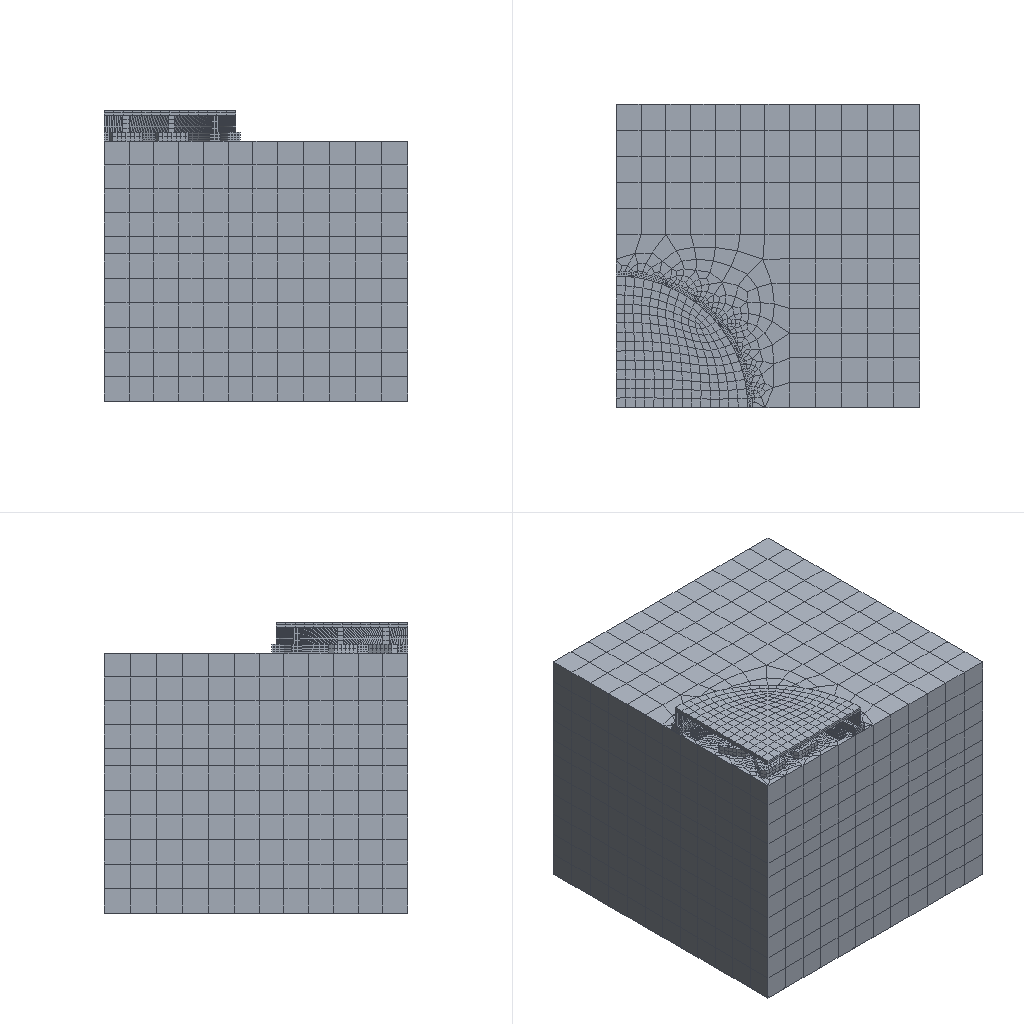Simulation study | abaqus
Set-up summary:
category,name,step,type,value,unit,region
solver,abaqus
solver,version,,,Abaqus/Standard 2020
units,not stated in the deck,,not stated
analysis,deck,,geostatic,geostatic
load_step,geo,geo,geostatic
load_step,load,load,static
load_step,requested,,,2
mesh,nodes,,,48393
mesh,elements,,,38413
element_type,C3D8,,solid,38413
load,load commands in deck,,count,2
bc,support commands in deck,,count,5
material,CANGDI,,in results
material,PILE,,in results
material,SOIL,,in results
check,setup vs results,,match,"per instance, exact: element labels, types and connectivity; labels of the nodes the elements use; coordinates of those nodes at SINGLE_PRECISION in 8 of 9 instance(s)"
Abaqus input file, long lists of numbers shortened:
*Heading
** Job name: Job-2 Model name: Model-1-4D-tiaoshi
** Generated by: Abaqus/CAE 2020
*Preprint, echo=NO, model=NO, history=NO, contact=NO
**
** PARTS
**
*Part, name=cangdi
*Node
      1,           0.,           0.,         0.25
      2,           0.,           0.,          0.5
** (637 more lines like these left out)
*Element, type=C3D8
  1,  72,  92, 320, 220,   1,   2,  22,  41
  2, 220, 320, 321, 221,  41,  22,  23,  40
** (372 more lines like these left out)
*Nset, nset=Set-1, generate
   1,  639,    1
*Elset, elset=Set-1, generate
   1,  374,    1
** Section: cangdi
*Solid Section, elset=Set-1, material=cangdi
,
*End Part
**
*Part, name=fangCT-Pile
*Node
      1,           0.,   1.2,           1.
      2,           0.,           0.,           1.
** (3217 more lines like these left out)
*Element, type=C3D8
   1,  266,  364,  282,  265, 1719, 1817, 1735, 1718
   2,  306,  289,   35,   34, 1759, 1742,  792,  793
** (2346 more lines like these left out)
*Nset, nset=Set-17, generate
    1,  3219,     1
*Elset, elset=Set-17, generate
    1,  2348,     1
** Section: pile
*Solid Section, elset=Set-17, material=pile
,
*End Part
**
*Part, name=huxingCT-pile
*Node
      1,   14.85,           0.,           3.
      2,           0.,   14.85,           3.
** (14026 more lines like these left out)
*Element, type=C3D8
  1,  494, 1649, 7421, 1647,    1,   65, 1423,  278
  2, 1649, 1650, 7422, 7421,   65,   66, 1424, 1423
** (10161 more lines like these left out)
*Nset, nset=Set-13, generate
     1,  14028,      1
*Elset, elset=Set-13, generate
     1,  10163,      1
** Section: pile
*Solid Section, elset=Set-13, material=pile
,
*End Part
**
*Part, name=sanjiaoCT-pile
*Node
      1,  0.35, -0.3489,           3.
      2, -0.35, -0.3489,           3.
** (776 more lines like these left out)
*Element, type=C3D8
1,  8,  5, 40, 41,  1,  2, 32, 37
2, 41, 40, 39, 42, 37, 32, 33, 36
** (366 more lines like these left out)
*Nset, nset=Set-5, generate
   1,  778,    1
*Elset, elset=Set-5, generate
   1,  368,    1
** Section: pile
*Solid Section, elset=Set-5, material=pile
,
*End Part
**
*Part, name=soil-1
*Node
      1,          20.,          20.,          39.
      2,           0.,          20.,          39.
** (24174 more lines like these left out)
*Element, type=C3D8
 1,   1,  81, 613, 100,   5, 101, 637, 120
 2,  81,  82, 614, 613, 101, 102, 638, 637
** (21706 more lines like these left out)
*Nset, nset=Set-4, generate
     1,  24176,      1
*Elset, elset=Set-4, generate
     1,  21708,      1
** Section: soil
*Solid Section, elset=Set-4, material=soil
,
*End Part
**
**
** ASSEMBLY
**
*Assembly, name=Assembly
**
*Instance, name=soil-1-1, part=soil-1
*End Instance
**
*Instance, name=cangdi-1, part=cangdi
          0.,           0.,          53.
*End Instance
**
*Instance, name=fangCT-Pile-3, part=fangCT-Pile
0.7,         12.2,          50.
*End Instance
**
*Instance, name=huxingCT-pile-1, part=huxingCT-pile
          0.,           0.,          50.
*End Instance
**
*Instance, name=sanjiaoCT-pile-5, part=sanjiaoCT-pile
         2.5,          2.5,          50.
*End Instance
**
*Instance, name=sanjiaoCT-pile-6, part=sanjiaoCT-pile
         7.8,          2.5,          50.
*End Instance
**
*Instance, name=sanjiaoCT-pile-7, part=sanjiaoCT-pile
2.5, 7.8,          50.
2.5, 7.8,          50., 2.5, 7.8,          51.,         180.
*End Instance
**
*Instance, name=sanjiaoCT-pile-8, part=sanjiaoCT-pile
         7.8,          7.8,          50.
         7.8,          7.8,          50.,          7.8,          7.8,          51.,         180.
*End Instance
**
*Instance, name=fangCT-Pile-4, part=fangCT-Pile
        12.2,          4.3,          50.
        12.2,          4.3,          50.,         12.2,          4.3, 49., 90.
*End Instance
**
*Node
      1,           6.,           6.,         56.5
*Nset, nset=Set-1
 1,
*Nset, nset=Set-2, instance=soil-1-1
   19,   20,   21,   22,   23,   24,   55,   56,   58,  207,  208,  209,  210,  211,  212,  213
  214,  239,  240,  241,  242,  243,  244,  245,  246,  247,  248,  447,  448,  449,  450,  451
** (3 more lines like these left out)
*Elset, elset=Set-2, instance=soil-1-1
   421,   422,   423,   424,   425,   456,   457,   458,   459,   460,   461,   462,   463,   464,   465,   466
   467,   468,   469,   470,   471,   472,   473,   474,   475,  1196,  1490,  1909,  1911,  1920,  2288,  2831
** (2 more lines like these left out)
*Nset, nset=Set-3, instance=soil-1-1
    2,    3,    6,    7,    9,   10,   11,   12,   20,   21,   24,   25,   30,   31,   32,   55
   56,   58,   87,   88,   89,   90,  107,  108,  109,  110,  129,  130,  131,  132,  141,  142
** (8 more lines like these left out)
*Elset, elset=Set-3, instance=soil-1-1
     7,    14,    21,    28,    35,    36,    41,    46,    51,    56,   425,   430,   435,   440,   445,   450
   455,   472,   473,   474,   475,   492,   493,   494,   495,   512,   513,   514,   515,   532,   533,   534
** (6 more lines like these left out)
*Nset, nset=Set-4, instance=soil-1-1
    3,    4,    7,    8,   10,   12,   19,   20,   21,   22,   23,   24,   29,   30,   31,   55
   56,   58,   91,   92,   93,   94,   95,   96,  111,  112,  113,  114,  115,  116,  125,  126
** (8 more lines like these left out)
*Elset, elset=Set-4, instance=soil-1-1
    29,    30,    31,    32,    33,    34,    35,    56,    57,    58,    59,    60,   421,   422,   423,   424
   425,   456,   457,   458,   459,   460,   461,   462,   463,   464,   465,   466,   467,   468,   469,   470
** (6 more lines like these left out)
*Nset, nset=Set-6
 1,
*Nset, nset=Set-7, instance=soil-1-1, generate
     1,  24176,      1
*Elset, elset=Set-7, instance=soil-1-1, generate
     1,  21708,      1
*Nset, nset=Set-10, instance=soil-1-1
    2,    3,    6,    7,    9,   10,   11,   12,   14,   15,   17,   18,   20,   21,   24,   25
   28,   30,   31,   32,   55,   56,   57,   58,   87,   88,   89,   90,  107,  108,  109,  110
** (18 more lines like these left out)
*Elset, elset=Set-10, instance=soil-1-1
     7,    14,    21,    28,    35,    36,    41,    46,    51,    56,    67,    74,    81,    88,    95,   102
   109,   116,   123,   130,   137,   144,   151,   158,   165,   172,   179,   186,   193,   200,   207,   214
** (15 more lines like these left out)
*Nset, nset=Set-11, instance=soil-1-1
    3,    4,    7,    8,   10,   12,   15,   16,   17,   19,   20,   21,   22,   23,   24,   27
   28,   29,   30,   31,   55,   56,   57,   58,   91,   92,   93,   94,   95,   96,  111,  112
** (18 more lines like these left out)
*Elset, elset=Set-11, instance=soil-1-1
    29,    30,    31,    32,    33,    34,    35,    56,    57,    58,    59,    60,    89,    90,    91,    92
    93,    94,    95,   124,   125,   126,   127,   128,   129,   130,   159,   160,   161,   162,   163,   164
** (15 more lines like these left out)
*Nset, nset=Set-12, instance=soil-1-1
   13,   14,   15,   16,   17,   18,   27,   28,   57,  145,  146,  147,  148,  149,  150,  151
  152,  153,  154,  155,  156,  157,  158,  159,  160,  161,  162,  163,  164,  185,  186,  187
** (125 more lines like these left out)
*Elset, elset=Set-12, instance=soil-1-1
    61,    62,    63,    64,    65,    66,    67,    68,    69,    70,    71,    72,    73,    74,    75,    76
    77,    78,    79,    80,    81,    82,    83,    84,    85,    86,    87,    88,    89,    90,    91,    92
** (123 more lines like these left out)
*Nset, nset=Set-13, instance=soil-1-1, generate
     1,  24176,      1
*Elset, elset=Set-13, instance=soil-1-1, generate
     1,  21708,      1
*Nset, nset=Set-14, instance=soil-1-1, generate
     1,  24176,      1
*Elset, elset=Set-14, instance=soil-1-1, generate
     1,  21708,      1
*Nset, nset=m_Set-9
 1,
*Elset, elset=_Surf-zhuding_S2, internal, instance=fangCT-Pile-3, generate
 1829,  1844,     1
*Elset, elset=_Surf-zhuding_S2, internal, instance=fangCT-Pile-4, generate
 1829,  1844,     1
*Elset, elset=_Surf-zhuding_S3, internal, instance=huxingCT-pile-1
   1,   2,   3,   4,   5,   6,   7,   8,   9,  10,  11,  12,  13,  14,  15,  16
  17,  18,  19,  20,  21,  22,  23,  24,  25,  26,  27,  28,  29,  30,  31,  32
** (13 more lines like these left out)
*Elset, elset=_Surf-zhuding_S3, internal, instance=sanjiaoCT-pile-7
 1,
*Elset, elset=_Surf-zhuding_S3, internal, instance=sanjiaoCT-pile-5
 1,
*Elset, elset=_Surf-zhuding_S3, internal, instance=sanjiaoCT-pile-8
 1,
*Elset, elset=_Surf-zhuding_S3, internal, instance=sanjiaoCT-pile-6
 1,
*Surface, type=ELEMENT, name=Surf-zhuding
_Surf-zhuding_S2, S2
_Surf-zhuding_S3, S3
*Elset, elset=_s_Surf-5_S4, internal, instance=cangdi-1, generate
   1,  121,    1
*Elset, elset=_s_Surf-5_S3, internal, instance=cangdi-1, generate
 122,  154,    1
*Elset, elset=_s_Surf-5_S2, internal, instance=cangdi-1, generate
 309,  341,    1
*Surface, type=ELEMENT, name=s_Surf-5
_s_Surf-5_S4, S4
_s_Surf-5_S3, S3
_s_Surf-5_S2, S2
*Elset, elset=_s_Surf-6_S2, internal, instance=soil-1-1, generate
 19863,  21708,      1
*Elset, elset=_s_Surf-6_S4, internal, instance=soil-1-1
 14332, 14347, 14366, 14367, 14381, 14388, 14389, 14427, 14443, 14465, 14472, 14484, 14504, 14515, 14516, 14523
 14531, 14559, 14581, 14596, 14602, 14693, 16178, 16193, 16212, 16213, 16227, 16234, 16235, 16273, 16289, 16311
** (4 more lines like these left out)
*Elset, elset=_s_Surf-6_S6, internal, instance=soil-1-1
 14331, 14352, 14369, 14371, 14372, 14376, 14380, 14382, 14393, 14406, 14407, 14415, 14418, 14449, 14452, 14469
 14475, 14477, 14487, 14506, 14509, 14513, 14519, 14522, 14524, 14601, 14626, 16177, 16198, 16215, 16217, 16218
** (5 more lines like these left out)
*Elset, elset=_s_Surf-6_S3, internal, instance=soil-1-1
 14326, 14354, 14363, 14379, 14390, 14400, 14413, 14433, 14462, 14463, 14534, 14545, 14557, 14570, 14577, 14584
 14620, 14632, 14640, 14656, 14669, 14672, 14679, 14698, 14915, 14944, 16172, 16200, 16209, 16225, 16236, 16246
** (5 more lines like these left out)
*Elset, elset=_s_Surf-6_S5, internal, instance=soil-1-1
 14335, 14343, 14359, 14361, 14365, 14370, 14386, 14391, 14395, 14403, 14421, 14423, 14425, 14431, 14451, 14453
 14466, 14470, 14473, 14478, 14482, 14483, 14486, 14488, 14491, 14498, 14499, 14501, 14507, 14510, 14514, 14518
** (13 more lines like these left out)
*Elset, elset=_s_Surf-6_S1, internal, instance=soil-1-1, generate
 1046,  1096,     1
*Surface, type=ELEMENT, name=s_Surf-6
_s_Surf-6_S2, S2
_s_Surf-6_S4, S4
_s_Surf-6_S6, S6
_s_Surf-6_S3, S3
_s_Surf-6_S5, S5
_s_Surf-6_S1, S1
*Elset, elset=_surf-allpile_S2, internal, instance=fangCT-Pile-3, generate
  871,  1044,     1
*Elset, elset=_surf-allpile_S2, internal, instance=huxingCT-pile-1, generate
 5325,  6287,     1
*Elset, elset=_surf-allpile_S2, internal, instance=sanjiaoCT-pile-7, generate
  55,  104,    1
*Elset, elset=_surf-allpile_S2, internal, instance=fangCT-Pile-4, generate
  871,  1044,     1
*Elset, elset=_surf-allpile_S2, internal, instance=sanjiaoCT-pile-5, generate
  55,  104,    1
*Elset, elset=_surf-allpile_S2, internal, instance=sanjiaoCT-pile-8, generate
  55,  104,    1
*Elset, elset=_surf-allpile_S2, internal, instance=sanjiaoCT-pile-6, generate
  55,  104,    1
*Surface, type=ELEMENT, name=surf-allpile
_surf-allpile_S2, S2
*Elset, elset=_surf-allsoil-p_S6, internal, instance=soil-1-1
   456,   460,   464,   468,   472,   476,   480,   484,   488,   492,   496,   500,   504,   508,   512,   516
   520,   524,   528,   532,   536,   540,   544,   548,   552,   556,   560,   564,   568,   572,   576,   580
** (10 more lines like these left out)
*Elset, elset=_surf-allsoil-p_S2, internal, instance=soil-1-1, generate
 19863,  21708,      1
*Elset, elset=_surf-allsoil-p_S4, internal, instance=soil-1-1
   809,   813,   817,   821,   825,   829,   833,   837,   841,   845,   849,   853,   857,   861,   865,   869
   873,   877,   881,   885,   889,   893,   897,   901,   905, 14332, 14347, 14366, 14367, 14381, 14388, 14389
** (6 more lines like these left out)
*Elset, elset=_surf-allsoil-p_S3, internal, instance=soil-1-1
 14326, 14354, 14363, 14379, 14390, 14400, 14413, 14433, 14462, 14463, 14534, 14545, 14557, 14570, 14577, 14584
 14620, 14632, 14640, 14656, 14669, 14672, 14679, 14698, 14915, 14944, 16172, 16200, 16209, 16225, 16236, 16246
** (5 more lines like these left out)
*Elset, elset=_surf-allsoil-p_S5, internal, instance=soil-1-1
 14335, 14343, 14359, 14361, 14365, 14370, 14386, 14391, 14395, 14403, 14421, 14423, 14425, 14431, 14451, 14453
 14466, 14470, 14473, 14478, 14482, 14483, 14486, 14488, 14491, 14498, 14499, 14501, 14507, 14510, 14514, 14518
** (13 more lines like these left out)
*Elset, elset=_surf-allsoil-p_S1, internal, instance=soil-1-1, generate
 1046,  1096,     1
*Surface, type=ELEMENT, name=surf-allsoil-p
_surf-allsoil-p_S6, S6
_surf-allsoil-p_S2, S2
_surf-allsoil-p_S4, S4
_surf-allsoil-p_S3, S3
_surf-allsoil-p_S5, S5
_surf-allsoil-p_S1, S1
*Elset, elset=_surf-cangdi_S4, internal, instance=cangdi-1, generate
 155,  187,    1
*Elset, elset=_surf-cangdi_S3, internal, instance=cangdi-1
 188, 189, 190, 191, 192, 193, 194, 195, 196, 197, 198, 199, 200, 201, 202, 203
 204, 205, 206, 207, 208, 209, 210, 211, 212, 213, 214, 215, 216, 217, 218, 219
** (8 more lines like these left out)
*Surface, type=ELEMENT, name=surf-cangdi
_surf-cangdi_S4, S4
_surf-cangdi_S3, S3
** Constraint: Constra-cang-zhu
*Tie, name=Constra-cang-zhu, adjust=yes
Surf-zhuding, surf-cangdi
** Constraint: Constraint-2
*Coupling, constraint name=Constraint-2, ref node=m_Set-9, surface=s_Surf-5
*Kinematic
*End Assembly
*Amplitude, name=Amp-1
             0.,              0.,              1.,              1.
**
** MATERIALS
**
*Material, name=cangdi
*Density
1000.,
*Elastic
 1e+11, 0.2
*Material, name=pile
*Density
1000.,
*Elastic
 3.7e+10, 0.17
*Material, name=soil
*Density
2000.,
*Elastic
 3e+07, 0.33
*Mohr Coulomb
35.,20.
*Mohr Coulomb Hardening
 1e+08,0.
**
** INTERACTION PROPERTIES
**
*Surface Interaction, name=moca
1.,
*Friction, slip tolerance=0.005
 0.3,
*Surface Behavior, pressure-overclosure=HARD
*Contact Damping, definition=DAMPING COEFFICIENT
0.2, 0.1, 0.
**
** BOUNDARY CONDITIONS
**
** Name: cankaodian Type: Displacement/Rotation
*Boundary
Set-6, 1, 1
Set-6, 2, 2
** Name: x Type: Displacement/Rotation
*Boundary
Set-10, 1, 1
** Name: y Type: Displacement/Rotation
*Boundary
Set-11, 2, 2
** Name: z Type: Displacement/Rotation
*Boundary
Set-12, 3, 3
**
** INTERACTIONS
**
** Interaction: pile-soil
*Contact Pair, interaction=moca, type=SURFACE TO SURFACE
s_Surf-6, surf-allpile
** ----------------------------------------------------------------
**
** STEP: geo
**
*Step, name=geo, nlgeom=YES, inc=10000, unsymm=YES
*Geostatic
**
** LOADS
**
** Name: Load-1   Type: Gravity
*Dload
, GRAV, 10., 0., 0., -1.
**
** OUTPUT REQUESTS
**
*Restart, write, frequency=0
**
** FIELD OUTPUT: F-Output-1
**
*Output, field, variable=PRESELECT
**
** HISTORY OUTPUT: H-Output-1
**
*Output, history, variable=PRESELECT
*End Step
** ----------------------------------------------------------------
**
** STEP: load
**
*Step, name=load, nlgeom=YES, inc=10000, unsymm=YES
*Static, stabilize=0.0002, allsdtol=0.05, continue=NO
0.001, 1., 1e-05, 1.
**
** LOADS
**
** Name: Load1   Type: Concentrated force
*Cload, amplitude=Amp-1
Set-1, 3, -5e+06
**
** OUTPUT REQUESTS
**
*Restart, write, frequency=0
**
** FIELD OUTPUT: F-Output-1
**
*Output, field
*Node Output
CF, RF, U, V
*Element Output, directions=YES
E, LE, MISES, PE, PEEQ, PEMAG, S
*Contact Output
CDISP, CSTRESS
**
** HISTORY OUTPUT: H-Output-1
**
*Output, history, variable=PRESELECT
*End Step
Results summary:
result,step,,completed,increments=1 time=1.0/1.0
result,step,,completed,increments=48 time=1.0/1.0
result,analysis,,,static
result,last_loadstep,,,2
result,primary field,,,U
result,reaction total,,FX,1555855.807,model units
result,reaction total,,FY,1555142.732,model units
result,reaction total,,FZ,736954337.65,model units